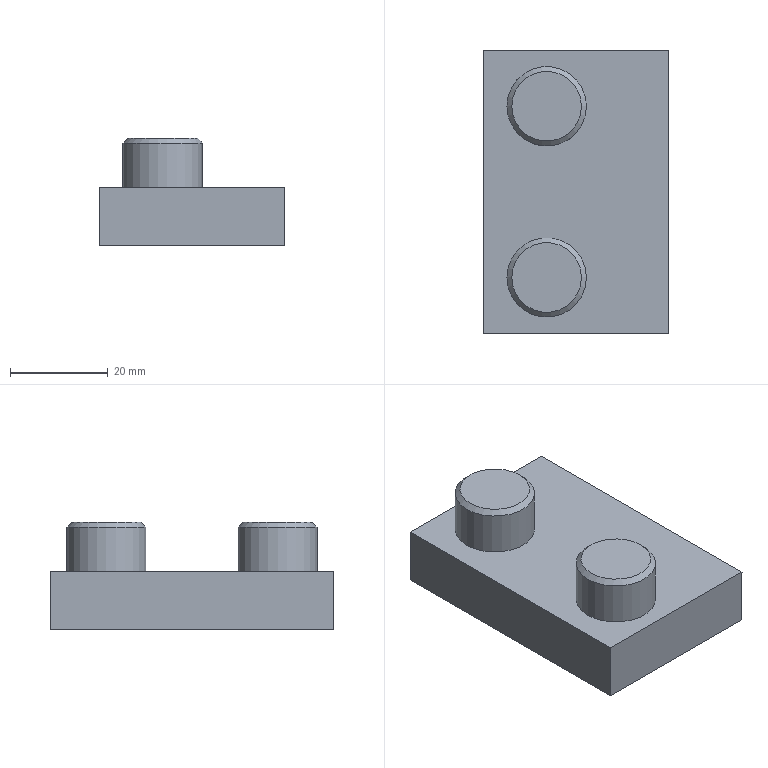Part | NX | features solid 2 | 1 solid | 12 faces | box 38 x 58 x 22 mm | volume 30547 mm3 | plane 8 | cylinder 2 | cone 2 | commonest cylinder face diameters 16.25 x2
STEP:
#1=CARTESIAN_POINT('',(-970.,414.,-108.));
#2=VERTEX_POINT('',#1);
#3=CARTESIAN_POINT('',(-1008.,414.,-108.));
#4=VERTEX_POINT('',#3);
#5=CARTESIAN_POINT('',(-970.,414.,-108.));
#6=CARTESIAN_POINT('',(-982.667,414.,-108.));
#7=CARTESIAN_POINT('',(-995.333,414.,-108.));
#8=CARTESIAN_POINT('',(-1008.,414.,-108.));
#9=B_SPLINE_CURVE_WITH_KNOTS('',3,(#5,#6,#7,#8),.UNSPECIFIED.,.F.,.F.,(4,4),(0.,1.),.UNSPECIFIED.);
#10=EDGE_CURVE('',#2,#4,#9,.T.);
#11=ORIENTED_EDGE('',*,*,#10,.F.);
#12=CARTESIAN_POINT('',(-970.,414.,-120.));
#13=VERTEX_POINT('',#12);
#14=CARTESIAN_POINT('',(-970.,414.,-120.));
#15=CARTESIAN_POINT('',(-970.,414.,-116.));
#16=CARTESIAN_POINT('',(-970.,414.,-112.));
#17=CARTESIAN_POINT('',(-970.,414.,-108.));
#18=B_SPLINE_CURVE_WITH_KNOTS('',3,(#14,#15,#16,#17),.UNSPECIFIED.,.F.,.F.,(4,4),(0.,1.),.UNSPECIFIED.);
#19=EDGE_CURVE('',#13,#2,#18,.T.);
#20=ORIENTED_EDGE('',*,*,#19,.F.);
#21=CARTESIAN_POINT('',(-1008.,414.,-120.));
#22=VERTEX_POINT('',#21);
#23=CARTESIAN_POINT('',(-1008.,414.,-120.));
#24=CARTESIAN_POINT('',(-995.333,414.,-120.));
#25=CARTESIAN_POINT('',(-982.667,414.,-120.));
#26=CARTESIAN_POINT('',(-970.,414.,-120.));
#27=B_SPLINE_CURVE_WITH_KNOTS('',3,(#23,#24,#25,#26),.UNSPECIFIED.,.F.,.F.,(4,4),(0.,1.),.UNSPECIFIED.);
#28=EDGE_CURVE('',#13,#22,#27,.F.);
#29=ORIENTED_EDGE('',*,*,#28,.T.);
#30=CARTESIAN_POINT('',(-1008.,414.,-108.));
#31=CARTESIAN_POINT('',(-1008.,414.,-112.));
#32=CARTESIAN_POINT('',(-1008.,414.,-116.));
#33=CARTESIAN_POINT('',(-1008.,414.,-120.));
#34=B_SPLINE_CURVE_WITH_KNOTS('',3,(#30,#31,#32,#33),.UNSPECIFIED.,.F.,.F.,(4,4),(0.,1.),.UNSPECIFIED.);
#35=EDGE_CURVE('',#22,#4,#34,.F.);
#36=ORIENTED_EDGE('',*,*,#35,.T.);
#37=EDGE_LOOP('',(#11,#20,#29,#36));
#38=FACE_BOUND('',#37,.T.);
#39=CARTESIAN_POINT('',(-989.,414.,-120.));
#40=DIRECTION('',(-0.000000011,1.,-0.00000017));
#41=DIRECTION('',(-0.000000341,-0.00000017,-1.));
#42=AXIS2_PLACEMENT_3D('',#39,#40,#41);
#43=PLANE('',#42);
#44=ADVANCED_FACE('',(#38),#43,.T.);
#45=CARTESIAN_POINT('',(-1008.,356.,-108.));
#46=VERTEX_POINT('',#45);
#47=CARTESIAN_POINT('',(-1008.,414.,-108.));
#48=CARTESIAN_POINT('',(-1008.,394.667,-108.));
#49=CARTESIAN_POINT('',(-1008.,375.333,-108.));
#50=CARTESIAN_POINT('',(-1008.,356.,-108.));
#51=B_SPLINE_CURVE_WITH_KNOTS('',3,(#47,#48,#49,#50),.UNSPECIFIED.,.F.,.F.,(4,4),(0.,1.),.UNSPECIFIED.);
#52=EDGE_CURVE('',#4,#46,#51,.T.);
#53=ORIENTED_EDGE('',*,*,#52,.F.);
#54=ORIENTED_EDGE('',*,*,#35,.F.);
#55=CARTESIAN_POINT('',(-1008.,356.,-120.));
#56=VERTEX_POINT('',#55);
#57=CARTESIAN_POINT('',(-1008.,356.,-120.));
#58=CARTESIAN_POINT('',(-1008.,375.333,-120.));
#59=CARTESIAN_POINT('',(-1008.,394.667,-120.));
#60=CARTESIAN_POINT('',(-1008.,414.,-120.));
#61=B_SPLINE_CURVE_WITH_KNOTS('',3,(#57,#58,#59,#60),.UNSPECIFIED.,.F.,.F.,(4,4),(0.,1.),.UNSPECIFIED.);
#62=EDGE_CURVE('',#22,#56,#61,.F.);
#63=ORIENTED_EDGE('',*,*,#62,.T.);
#64=CARTESIAN_POINT('',(-1008.,356.,-108.));
#65=CARTESIAN_POINT('',(-1008.,356.,-112.));
#66=CARTESIAN_POINT('',(-1008.,356.,-116.));
#67=CARTESIAN_POINT('',(-1008.,356.,-120.));
#68=B_SPLINE_CURVE_WITH_KNOTS('',3,(#64,#65,#66,#67),.UNSPECIFIED.,.F.,.F.,(4,4),(0.,1.),.UNSPECIFIED.);
#69=EDGE_CURVE('',#56,#46,#68,.F.);
#70=ORIENTED_EDGE('',*,*,#69,.T.);
#71=EDGE_LOOP('',(#53,#54,#63,#70));
#72=FACE_BOUND('',#71,.T.);
#73=CARTESIAN_POINT('',(-1008.,385.,-120.));
#74=DIRECTION('',(-1.,-0.000000011,0.000000341));
#75=DIRECTION('',(-0.000000341,-0.00000017,-1.));
#76=AXIS2_PLACEMENT_3D('',#73,#74,#75);
#77=PLANE('',#76);
#78=ADVANCED_FACE('',(#72),#77,.T.);
#79=CARTESIAN_POINT('',(-970.,356.,-108.));
#80=VERTEX_POINT('',#79);
#81=CARTESIAN_POINT('',(-1008.,356.,-108.));
#82=CARTESIAN_POINT('',(-995.333,356.,-108.));
#83=CARTESIAN_POINT('',(-982.667,356.,-108.));
#84=CARTESIAN_POINT('',(-970.,356.,-108.));
#85=B_SPLINE_CURVE_WITH_KNOTS('',3,(#81,#82,#83,#84),.UNSPECIFIED.,.F.,.F.,(4,4),(0.,1.),.UNSPECIFIED.);
#86=EDGE_CURVE('',#46,#80,#85,.T.);
#87=ORIENTED_EDGE('',*,*,#86,.F.);
#88=ORIENTED_EDGE('',*,*,#69,.F.);
#89=CARTESIAN_POINT('',(-970.,356.,-120.));
#90=VERTEX_POINT('',#89);
#91=CARTESIAN_POINT('',(-970.,356.,-120.));
#92=CARTESIAN_POINT('',(-982.667,356.,-120.));
#93=CARTESIAN_POINT('',(-995.333,356.,-120.));
#94=CARTESIAN_POINT('',(-1008.,356.,-120.));
#95=B_SPLINE_CURVE_WITH_KNOTS('',3,(#91,#92,#93,#94),.UNSPECIFIED.,.F.,.F.,(4,4),(0.,1.),.UNSPECIFIED.);
#96=EDGE_CURVE('',#56,#90,#95,.F.);
#97=ORIENTED_EDGE('',*,*,#96,.T.);
#98=CARTESIAN_POINT('',(-970.,356.,-108.));
#99=CARTESIAN_POINT('',(-970.,356.,-112.));
#100=CARTESIAN_POINT('',(-970.,356.,-116.));
#101=CARTESIAN_POINT('',(-970.,356.,-120.));
#102=B_SPLINE_CURVE_WITH_KNOTS('',3,(#98,#99,#100,#101),.UNSPECIFIED.,.F.,.F.,(4,4),(0.,1.),.UNSPECIFIED.);
#103=EDGE_CURVE('',#90,#80,#102,.F.);
#104=ORIENTED_EDGE('',*,*,#103,.T.);
#105=EDGE_LOOP('',(#87,#88,#97,#104));
#106=FACE_BOUND('',#105,.T.);
#107=CARTESIAN_POINT('',(-989.,356.,-120.));
#108=DIRECTION('',(0.000000011,-1.,0.00000017));
#109=DIRECTION('',(0.000000341,0.00000017,1.));
#110=AXIS2_PLACEMENT_3D('',#107,#108,#109);
#111=PLANE('',#110);
#112=ADVANCED_FACE('',(#106),#111,.T.);
#113=CARTESIAN_POINT('',(-970.,356.,-108.));
#114=CARTESIAN_POINT('',(-970.,375.333,-108.));
#115=CARTESIAN_POINT('',(-970.,394.667,-108.));
#116=CARTESIAN_POINT('',(-970.,414.,-108.));
#117=B_SPLINE_CURVE_WITH_KNOTS('',3,(#113,#114,#115,#116),.UNSPECIFIED.,.F.,.F.,(4,4),(0.,1.),.UNSPECIFIED.);
#118=EDGE_CURVE('',#80,#2,#117,.T.);
#119=ORIENTED_EDGE('',*,*,#118,.F.);
#120=ORIENTED_EDGE('',*,*,#103,.F.);
#121=CARTESIAN_POINT('',(-970.,414.,-120.));
#122=CARTESIAN_POINT('',(-970.,394.667,-120.));
#123=CARTESIAN_POINT('',(-970.,375.333,-120.));
#124=CARTESIAN_POINT('',(-970.,356.,-120.));
#125=B_SPLINE_CURVE_WITH_KNOTS('',3,(#121,#122,#123,#124),.UNSPECIFIED.,.F.,.F.,(4,4),(0.,1.),.UNSPECIFIED.);
#126=EDGE_CURVE('',#90,#13,#125,.F.);
#127=ORIENTED_EDGE('',*,*,#126,.T.);
#128=ORIENTED_EDGE('',*,*,#19,.T.);
#129=EDGE_LOOP('',(#119,#120,#127,#128));
#130=FACE_BOUND('',#129,.T.);
#131=CARTESIAN_POINT('',(-970.,385.,-120.));
#132=DIRECTION('',(1.,0.000000011,-0.000000341));
#133=DIRECTION('',(0.000000341,0.00000017,1.));
#134=AXIS2_PLACEMENT_3D('',#131,#132,#133);
#135=PLANE('',#134);
#136=ADVANCED_FACE('',(#130),#135,.T.);
#137=ORIENTED_EDGE('',*,*,#28,.F.);
#138=ORIENTED_EDGE('',*,*,#126,.F.);
#139=ORIENTED_EDGE('',*,*,#96,.F.);
#140=ORIENTED_EDGE('',*,*,#62,.F.);
#141=EDGE_LOOP('',(#137,#138,#139,#140));
#142=FACE_BOUND('',#141,.T.);
#143=CARTESIAN_POINT('',(-989.,385.,-120.));
#144=DIRECTION('',(0.000000341,0.00000017,1.));
#145=DIRECTION('',(0.000000011,-1.,0.00000017));
#146=AXIS2_PLACEMENT_3D('',#143,#144,#145);
#147=PLANE('',#146);
#148=ADVANCED_FACE('',(#142),#147,.F.);
#149=CARTESIAN_POINT('',(-1003.125,367.5,-108.));
#150=VERTEX_POINT('',#149);
#151=CARTESIAN_POINT('',(-995.,367.5,-108.));
#152=DIRECTION('',(0.000000341,0.00000017,1.));
#153=DIRECTION('',(-1.,-0.000000011,0.000000341));
#154=AXIS2_PLACEMENT_3D('',#151,#152,#153);
#155=CIRCLE('',#154,8.125);
#156=EDGE_CURVE('',#150,#150,#155,.T.);
#157=ORIENTED_EDGE('',*,*,#156,.F.);
#158=EDGE_LOOP('',(#157));
#159=FACE_BOUND('',#158,.T.);
#160=CARTESIAN_POINT('',(-1003.125,402.5,-108.));
#161=VERTEX_POINT('',#160);
#162=CARTESIAN_POINT('',(-995.,402.5,-108.));
#163=DIRECTION('',(0.000000341,0.00000017,1.));
#164=DIRECTION('',(-1.,-0.000000011,0.000000341));
#165=AXIS2_PLACEMENT_3D('',#162,#163,#164);
#166=CIRCLE('',#165,8.125);
#167=EDGE_CURVE('',#161,#161,#166,.T.);
#168=ORIENTED_EDGE('',*,*,#167,.F.);
#169=EDGE_LOOP('',(#168));
#170=FACE_BOUND('',#169,.T.);
#171=ORIENTED_EDGE('',*,*,#10,.T.);
#172=ORIENTED_EDGE('',*,*,#52,.T.);
#173=ORIENTED_EDGE('',*,*,#86,.T.);
#174=ORIENTED_EDGE('',*,*,#118,.T.);
#175=EDGE_LOOP('',(#171,#172,#173,#174));
#176=FACE_BOUND('',#175,.T.);
#177=CARTESIAN_POINT('',(-989.,385.,-108.));
#178=DIRECTION('',(0.000000341,0.00000017,1.));
#179=DIRECTION('',(0.000000011,-1.,0.00000017));
#180=AXIS2_PLACEMENT_3D('',#177,#178,#179);
#181=PLANE('',#180);
#182=ADVANCED_FACE('',(#159,#170,#176),#181,.T.);
#183=CARTESIAN_POINT('',(-1002.125,402.5,-98.));
#184=VERTEX_POINT('',#183);
#185=CARTESIAN_POINT('',(-995.,402.5,-98.));
#186=DIRECTION('',(0.000000341,0.00000017,1.));
#187=DIRECTION('',(-1.,-0.000000011,0.000000341));
#188=AXIS2_PLACEMENT_3D('',#185,#186,#187);
#189=CIRCLE('',#188,7.125);
#190=EDGE_CURVE('',#184,#184,#189,.T.);
#191=ORIENTED_EDGE('',*,*,#190,.T.);
#192=EDGE_LOOP('',(#191));
#193=FACE_BOUND('',#192,.T.);
#194=CARTESIAN_POINT('',(-995.,402.5,-98.));
#195=DIRECTION('',(0.000000341,0.00000017,1.));
#196=DIRECTION('',(-1.,-0.000000011,0.000000341));
#197=AXIS2_PLACEMENT_3D('',#194,#195,#196);
#198=PLANE('',#197);
#199=ADVANCED_FACE('',(#193),#198,.T.);
#200=CARTESIAN_POINT('',(-1003.125,402.5,-99.));
#201=VERTEX_POINT('',#200);
#202=CARTESIAN_POINT('',(-995.,402.5,-99.));
#203=DIRECTION('',(0.000000341,0.00000017,1.));
#204=DIRECTION('',(-1.,-0.000000011,0.000000341));
#205=AXIS2_PLACEMENT_3D('',#202,#203,#204);
#206=CIRCLE('',#205,8.125);
#207=EDGE_CURVE('',#201,#201,#206,.F.);
#208=ORIENTED_EDGE('',*,*,#207,.T.);
#209=EDGE_LOOP('',(#208));
#210=FACE_BOUND('',#209,.T.);
#211=ORIENTED_EDGE('',*,*,#167,.T.);
#212=EDGE_LOOP('',(#211));
#213=FACE_BOUND('',#212,.T.);
#214=CARTESIAN_POINT('',(-995.,402.5,-108.));
#215=DIRECTION('',(0.000000341,0.00000017,1.));
#216=DIRECTION('',(-1.,-0.000000011,0.000000341));
#217=AXIS2_PLACEMENT_3D('',#214,#215,#216);
#218=CYLINDRICAL_SURFACE('',#217,8.125);
#219=ADVANCED_FACE('',(#210,#213),#218,.T.);
#220=CARTESIAN_POINT('',(-1002.125,367.5,-98.));
#221=VERTEX_POINT('',#220);
#222=CARTESIAN_POINT('',(-995.,367.5,-98.));
#223=DIRECTION('',(0.000000341,0.00000017,1.));
#224=DIRECTION('',(-1.,-0.000000011,0.000000341));
#225=AXIS2_PLACEMENT_3D('',#222,#223,#224);
#226=CIRCLE('',#225,7.125);
#227=EDGE_CURVE('',#221,#221,#226,.T.);
#228=ORIENTED_EDGE('',*,*,#227,.T.);
#229=EDGE_LOOP('',(#228));
#230=FACE_BOUND('',#229,.T.);
#231=CARTESIAN_POINT('',(-995.,367.5,-98.));
#232=DIRECTION('',(0.000000341,0.00000017,1.));
#233=DIRECTION('',(-1.,-0.000000011,0.000000341));
#234=AXIS2_PLACEMENT_3D('',#231,#232,#233);
#235=PLANE('',#234);
#236=ADVANCED_FACE('',(#230),#235,.T.);
#237=CARTESIAN_POINT('',(-1003.125,367.5,-99.));
#238=VERTEX_POINT('',#237);
#239=CARTESIAN_POINT('',(-995.,367.5,-99.));
#240=DIRECTION('',(0.000000341,0.00000017,1.));
#241=DIRECTION('',(-1.,-0.000000011,0.000000341));
#242=AXIS2_PLACEMENT_3D('',#239,#240,#241);
#243=CIRCLE('',#242,8.125);
#244=EDGE_CURVE('',#238,#238,#243,.F.);
#245=ORIENTED_EDGE('',*,*,#244,.T.);
#246=EDGE_LOOP('',(#245));
#247=FACE_BOUND('',#246,.T.);
#248=ORIENTED_EDGE('',*,*,#156,.T.);
#249=EDGE_LOOP('',(#248));
#250=FACE_BOUND('',#249,.T.);
#251=CARTESIAN_POINT('',(-995.,367.5,-108.));
#252=DIRECTION('',(0.000000341,0.00000017,1.));
#253=DIRECTION('',(-1.,-0.000000011,0.000000341));
#254=AXIS2_PLACEMENT_3D('',#251,#252,#253);
#255=CYLINDRICAL_SURFACE('',#254,8.125);
#256=ADVANCED_FACE('',(#247,#250),#255,.T.);
#257=ORIENTED_EDGE('',*,*,#244,.F.);
#258=EDGE_LOOP('',(#257));
#259=FACE_BOUND('',#258,.T.);
#260=ORIENTED_EDGE('',*,*,#227,.F.);
#261=EDGE_LOOP('',(#260));
#262=FACE_BOUND('',#261,.T.);
#263=CARTESIAN_POINT('',(-995.,367.5,-98.));
#264=DIRECTION('',(-0.000000341,-0.00000017,-1.));
#265=DIRECTION('',(1.,0.000000011,-0.000000341));
#266=AXIS2_PLACEMENT_3D('',#263,#264,#265);
#267=CONICAL_SURFACE('',#266,7.125,0.7854);
#268=ADVANCED_FACE('',(#259,#262),#267,.T.);
#269=ORIENTED_EDGE('',*,*,#207,.F.);
#270=EDGE_LOOP('',(#269));
#271=FACE_BOUND('',#270,.T.);
#272=ORIENTED_EDGE('',*,*,#190,.F.);
#273=EDGE_LOOP('',(#272));
#274=FACE_BOUND('',#273,.T.);
#275=CARTESIAN_POINT('',(-995.,402.5,-98.));
#276=DIRECTION('',(-0.000000341,-0.00000017,-1.));
#277=DIRECTION('',(1.,0.000000011,-0.000000341));
#278=AXIS2_PLACEMENT_3D('',#275,#276,#277);
#279=CONICAL_SURFACE('',#278,7.125,0.7854);
#280=ADVANCED_FACE('',(#271,#274),#279,.T.);
#281=CLOSED_SHELL('',(#44,#78,#112,#136,#148,#182,#199,#219,#236,#256,#268,#280));
#282=MANIFOLD_SOLID_BREP('',#281);
#283=(LENGTH_UNIT()NAMED_UNIT(*)SI_UNIT(.MILLI.,.METRE.));
#284=UNCERTAINTY_MEASURE_WITH_UNIT(LENGTH_MEASURE(0.0508),#283,'','');
#285=(NAMED_UNIT(*)PLANE_ANGLE_UNIT()SI_UNIT($,.RADIAN.));
#286=(NAMED_UNIT(*)SI_UNIT($,.STERADIAN.)SOLID_ANGLE_UNIT());
#287=(GEOMETRIC_REPRESENTATION_CONTEXT(3)GLOBAL_UNCERTAINTY_ASSIGNED_CONTEXT((#284))GLOBAL_UNIT_ASSIGNED_CONTEXT((#283,#285,#286))REPRESENTATION_CONTEXT('',''));
#288=ADVANCED_BREP_SHAPE_REPRESENTATION('',(#282),#287);